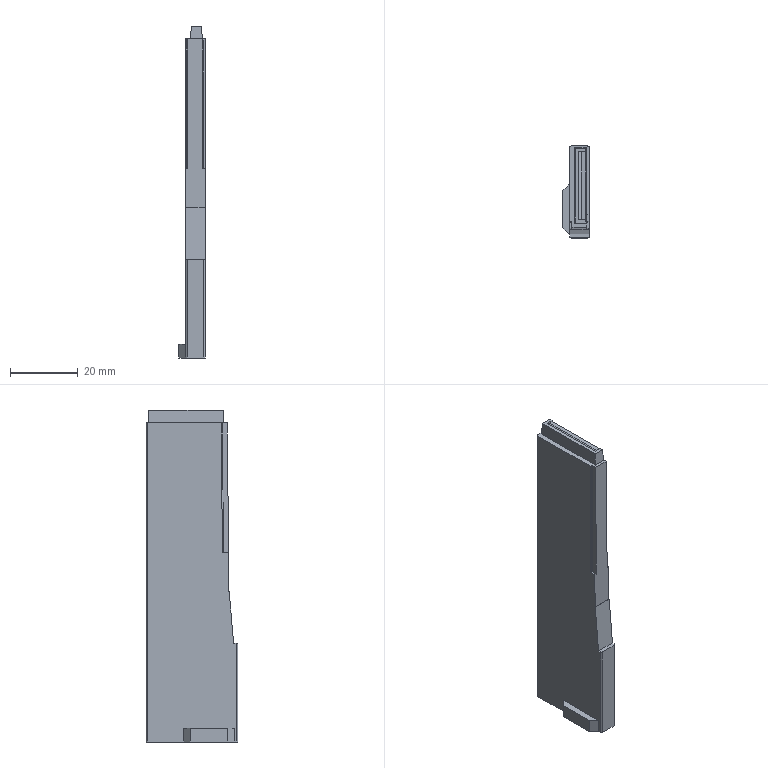Part | Creo | 1 solid | 40 faces | box 7.8 x 27 x 97.99 mm | volume 14019 mm3 | plane 33 | cylinder 7 | commonest cylinder face diameters 1 x4 0.603 x3
STEP:
#1=CARTESIAN_POINT('',(0.,0.,0.));
#2=DIRECTION('',(0.,0.,1.));
#3=DIRECTION('',(1.,0.,0.));
#4=AXIS2_PLACEMENT_3D('',#1,#2,#3);
#5=CARTESIAN_POINT('',(15.65,-83.325,43.9));
#6=VERTEX_POINT('',#5);
#7=CARTESIAN_POINT('',(15.65,-63.225,43.9));
#8=VERTEX_POINT('',#7);
#9=CARTESIAN_POINT('',(15.65,-83.325,43.9));
#10=DIRECTION('',(0.,1.,0.));
#11=VECTOR('',#10,20.1);
#12=LINE('',#9,#11);
#13=EDGE_CURVE('',#6,#8,#12,.T.);
#14=ORIENTED_EDGE('',*,*,#13,.T.);
#15=CARTESIAN_POINT('',(16.566,-63.256,43.548));
#16=VERTEX_POINT('',#15);
#17=CARTESIAN_POINT('',(15.65,-63.225,43.9));
#18=DIRECTION('',(0.9329,-0.03139,-0.3588));
#19=VECTOR('',#18,0.9817);
#20=LINE('',#17,#19);
#21=EDGE_CURVE('',#8,#16,#20,.T.);
#22=ORIENTED_EDGE('',*,*,#21,.T.);
#23=CARTESIAN_POINT('',(16.566,-83.294,43.548));
#24=VERTEX_POINT('',#23);
#25=CARTESIAN_POINT('',(16.566,-83.294,43.548));
#26=DIRECTION('',(0.,1.,0.));
#27=VECTOR('',#26,20.038);
#28=LINE('',#25,#27);
#29=EDGE_CURVE('',#24,#16,#28,.T.);
#30=ORIENTED_EDGE('',*,*,#29,.F.);
#31=CARTESIAN_POINT('',(15.65,-83.325,43.9));
#32=DIRECTION('',(0.9329,0.03139,-0.3588));
#33=VECTOR('',#32,0.9817);
#34=LINE('',#31,#33);
#35=EDGE_CURVE('',#6,#24,#34,.T.);
#36=ORIENTED_EDGE('',*,*,#35,.F.);
#37=EDGE_LOOP('',(#14,#22,#30,#36));
#38=FACE_OUTER_BOUND('',#37,.F.);
#39=CARTESIAN_POINT('',(15.65,-83.325,43.9));
#40=DIRECTION('',(-0.359,0.,-0.9333));
#41=DIRECTION('',(-0.9333,0.,0.359));
#42=AXIS2_PLACEMENT_3D('',#39,#40,#41);
#43=PLANE('',#42);
#44=ADVANCED_FACE('',(#38),#43,.F.);
#45=CARTESIAN_POINT('',(17.723,-62.246,43.9));
#46=VERTEX_POINT('',#45);
#47=CARTESIAN_POINT('',(14.671,-62.246,43.9));
#48=VERTEX_POINT('',#47);
#49=CARTESIAN_POINT('',(17.723,-62.246,43.9));
#50=DIRECTION('',(-1.,0.,0.));
#51=VECTOR('',#50,3.052);
#52=LINE('',#49,#51);
#53=EDGE_CURVE('',#46,#48,#52,.T.);
#54=ORIENTED_EDGE('',*,*,#53,.F.);
#55=CARTESIAN_POINT('',(17.723,-63.225,43.9));
#56=VERTEX_POINT('',#55);
#57=CARTESIAN_POINT('',(17.723,-63.225,43.9));
#58=DIRECTION('',(0.,1.,0.));
#59=VECTOR('',#58,0.9787);
#60=LINE('',#57,#59);
#61=EDGE_CURVE('',#56,#46,#60,.T.);
#62=ORIENTED_EDGE('',*,*,#61,.F.);
#63=CARTESIAN_POINT('',(15.65,-63.225,43.9));
#64=DIRECTION('',(1.,0.,0.));
#65=VECTOR('',#64,2.073);
#66=LINE('',#63,#65);
#67=EDGE_CURVE('',#8,#56,#66,.T.);
#68=ORIENTED_EDGE('',*,*,#67,.F.);
#69=ORIENTED_EDGE('',*,*,#13,.F.);
#70=CARTESIAN_POINT('',(17.723,-83.325,43.9));
#71=VERTEX_POINT('',#70);
#72=CARTESIAN_POINT('',(15.65,-83.325,43.9));
#73=DIRECTION('',(1.,0.,0.));
#74=VECTOR('',#73,2.073);
#75=LINE('',#72,#74);
#76=EDGE_CURVE('',#6,#71,#75,.T.);
#77=ORIENTED_EDGE('',*,*,#76,.T.);
#78=CARTESIAN_POINT('',(17.723,-84.304,43.9));
#79=VERTEX_POINT('',#78);
#80=CARTESIAN_POINT('',(17.723,-84.304,43.9));
#81=DIRECTION('',(0.,1.,0.));
#82=VECTOR('',#81,0.9787);
#83=LINE('',#80,#82);
#84=EDGE_CURVE('',#79,#71,#83,.T.);
#85=ORIENTED_EDGE('',*,*,#84,.F.);
#86=CARTESIAN_POINT('',(14.671,-84.304,43.9));
#87=VERTEX_POINT('',#86);
#88=CARTESIAN_POINT('',(14.671,-84.304,43.9));
#89=DIRECTION('',(1.,0.,0.));
#90=VECTOR('',#89,3.052);
#91=LINE('',#88,#90);
#92=EDGE_CURVE('',#87,#79,#91,.T.);
#93=ORIENTED_EDGE('',*,*,#92,.F.);
#94=CARTESIAN_POINT('',(14.671,-62.246,43.9));
#95=DIRECTION('',(0.,-1.,0.));
#96=VECTOR('',#95,22.057);
#97=LINE('',#94,#96);
#98=EDGE_CURVE('',#48,#87,#97,.T.);
#99=ORIENTED_EDGE('',*,*,#98,.F.);
#100=EDGE_LOOP('',(#54,#62,#68,#69,#77,#85,#93,#99));
#101=FACE_OUTER_BOUND('',#100,.F.);
#102=CARTESIAN_POINT('',(-46.35,-83.325,43.9));
#103=DIRECTION('',(0.,0.,-1.));
#104=DIRECTION('',(0.,-1.,0.));
#105=AXIS2_PLACEMENT_3D('',#102,#103,#104);
#106=PLANE('',#105);
#107=ADVANCED_FACE('',(#101),#106,.F.);
#108=CARTESIAN_POINT('',(17.722,-62.245,43.876));
#109=VERTEX_POINT('',#108);
#110=CARTESIAN_POINT('',(17.722,-62.245,43.876));
#111=DIRECTION('',(0.03485,-0.0523,0.998));
#112=VECTOR('',#111,0.02412);
#113=LINE('',#110,#112);
#114=EDGE_CURVE('',#109,#46,#113,.T.);
#115=ORIENTED_EDGE('',*,*,#114,.T.);
#116=ORIENTED_EDGE('',*,*,#53,.T.);
#117=CARTESIAN_POINT('',(14.471,-62.046,40.081));
#118=VERTEX_POINT('',#117);
#119=CARTESIAN_POINT('',(14.671,-62.246,43.9));
#120=DIRECTION('',(-0.05226,0.05226,-0.9973));
#121=VECTOR('',#120,3.829);
#122=LINE('',#119,#121);
#123=EDGE_CURVE('',#48,#118,#122,.T.);
#124=ORIENTED_EDGE('',*,*,#123,.T.);
#125=CARTESIAN_POINT('',(17.921,-62.046,40.081));
#126=VERTEX_POINT('',#125);
#127=CARTESIAN_POINT('',(14.471,-62.046,40.081));
#128=DIRECTION('',(1.,0.,0.));
#129=VECTOR('',#128,3.45);
#130=LINE('',#127,#129);
#131=EDGE_CURVE('',#118,#126,#130,.T.);
#132=ORIENTED_EDGE('',*,*,#131,.T.);
#133=CARTESIAN_POINT('',(17.921,-62.046,40.081));
#134=DIRECTION('',(-0.05226,-0.05226,0.9973));
#135=VECTOR('',#134,3.805);
#136=LINE('',#133,#135);
#137=EDGE_CURVE('',#126,#109,#136,.T.);
#138=ORIENTED_EDGE('',*,*,#137,.T.);
#139=EDGE_LOOP('',(#115,#116,#124,#132,#138));
#140=FACE_OUTER_BOUND('',#139,.F.);
#141=CARTESIAN_POINT('',(21.275,-62.22,43.398));
#142=DIRECTION('',(0.,0.9986,0.05234));
#143=DIRECTION('',(-1.,0.,0.));
#144=AXIS2_PLACEMENT_3D('',#141,#142,#143);
#145=PLANE('',#144);
#146=ADVANCED_FACE('',(#140),#145,.T.);
#147=ORIENTED_EDGE('',*,*,#61,.T.);
#148=ORIENTED_EDGE('',*,*,#114,.F.);
#149=CARTESIAN_POINT('',(17.722,-63.227,43.876));
#150=VERTEX_POINT('',#149);
#151=CARTESIAN_POINT('',(17.722,-63.227,43.876));
#152=DIRECTION('',(0.,1.,0.));
#153=VECTOR('',#152,0.982);
#154=LINE('',#151,#153);
#155=EDGE_CURVE('',#150,#109,#154,.T.);
#156=ORIENTED_EDGE('',*,*,#155,.F.);
#157=CARTESIAN_POINT('',(17.723,-63.225,43.9));
#158=DIRECTION('',(-0.03477,-0.0871,-0.9956));
#159=VECTOR('',#158,0.02417);
#160=LINE('',#157,#159);
#161=EDGE_CURVE('',#56,#150,#160,.T.);
#162=ORIENTED_EDGE('',*,*,#161,.F.);
#163=EDGE_LOOP('',(#147,#148,#156,#162));
#164=FACE_OUTER_BOUND('',#163,.F.);
#165=CARTESIAN_POINT('',(17.66,-62.152,42.091));
#166=DIRECTION('',(-0.9994,0.,0.0349));
#167=DIRECTION('',(0.0349,0.,0.9994));
#168=AXIS2_PLACEMENT_3D('',#165,#166,#167);
#169=PLANE('',#168);
#170=ADVANCED_FACE('',(#164),#169,.F.);
#171=CARTESIAN_POINT('',(17.74,-83.294,43.548));
#172=VERTEX_POINT('',#171);
#173=CARTESIAN_POINT('',(17.74,-63.256,43.548));
#174=VERTEX_POINT('',#173);
#175=CARTESIAN_POINT('',(17.74,-83.294,43.548));
#176=DIRECTION('',(0.,1.,0.));
#177=VECTOR('',#176,20.038);
#178=LINE('',#175,#177);
#179=EDGE_CURVE('',#172,#174,#178,.T.);
#180=ORIENTED_EDGE('',*,*,#179,.T.);
#181=CARTESIAN_POINT('',(17.722,-63.227,43.876));
#182=DIRECTION('',(0.05214,-0.08704,-0.9948));
#183=VECTOR('',#182,0.3299);
#184=LINE('',#181,#183);
#185=EDGE_CURVE('',#150,#174,#184,.T.);
#186=ORIENTED_EDGE('',*,*,#185,.F.);
#187=ORIENTED_EDGE('',*,*,#155,.T.);
#188=ORIENTED_EDGE('',*,*,#137,.F.);
#189=CARTESIAN_POINT('',(17.921,-84.504,40.081));
#190=VERTEX_POINT('',#189);
#191=CARTESIAN_POINT('',(17.921,-84.504,40.081));
#192=DIRECTION('',(0.,1.,0.));
#193=VECTOR('',#192,22.458);
#194=LINE('',#191,#193);
#195=EDGE_CURVE('',#190,#126,#194,.T.);
#196=ORIENTED_EDGE('',*,*,#195,.F.);
#197=CARTESIAN_POINT('',(17.722,-84.305,43.876));
#198=VERTEX_POINT('',#197);
#199=CARTESIAN_POINT('',(17.722,-84.305,43.876));
#200=DIRECTION('',(0.05226,-0.05226,-0.9973));
#201=VECTOR('',#200,3.805);
#202=LINE('',#199,#201);
#203=EDGE_CURVE('',#198,#190,#202,.T.);
#204=ORIENTED_EDGE('',*,*,#203,.F.);
#205=CARTESIAN_POINT('',(17.722,-83.323,43.876));
#206=VERTEX_POINT('',#205);
#207=CARTESIAN_POINT('',(17.722,-84.305,43.876));
#208=DIRECTION('',(0.,1.,0.));
#209=VECTOR('',#208,0.982);
#210=LINE('',#207,#209);
#211=EDGE_CURVE('',#198,#206,#210,.T.);
#212=ORIENTED_EDGE('',*,*,#211,.T.);
#213=CARTESIAN_POINT('',(17.74,-83.294,43.548));
#214=DIRECTION('',(-0.05214,-0.08704,0.9948));
#215=VECTOR('',#214,0.3299);
#216=LINE('',#213,#215);
#217=EDGE_CURVE('',#172,#206,#216,.T.);
#218=ORIENTED_EDGE('',*,*,#217,.F.);
#219=EDGE_LOOP('',(#180,#186,#187,#188,#196,#204,#212,#218));
#220=FACE_OUTER_BOUND('',#219,.F.);
#221=CARTESIAN_POINT('',(17.747,-90.96,43.402));
#222=DIRECTION('',(-0.9986,0.,-0.05234));
#223=DIRECTION('',(0.,-1.,0.));
#224=AXIS2_PLACEMENT_3D('',#221,#222,#223);
#225=PLANE('',#224);
#226=ADVANCED_FACE('',(#220),#225,.F.);
#227=ORIENTED_EDGE('',*,*,#29,.T.);
#228=CARTESIAN_POINT('',(16.566,-63.256,43.548));
#229=DIRECTION('',(1.,0.,0.));
#230=VECTOR('',#229,1.174);
#231=LINE('',#228,#230);
#232=EDGE_CURVE('',#16,#174,#231,.T.);
#233=ORIENTED_EDGE('',*,*,#232,.T.);
#234=ORIENTED_EDGE('',*,*,#179,.F.);
#235=CARTESIAN_POINT('',(16.566,-83.294,43.548));
#236=DIRECTION('',(1.,0.,0.));
#237=VECTOR('',#236,1.174);
#238=LINE('',#235,#237);
#239=EDGE_CURVE('',#24,#172,#238,.T.);
#240=ORIENTED_EDGE('',*,*,#239,.F.);
#241=EDGE_LOOP('',(#227,#233,#234,#240));
#242=FACE_OUTER_BOUND('',#241,.F.);
#243=CARTESIAN_POINT('',(16.956,-83.325,43.548));
#244=DIRECTION('',(0.,0.,-1.));
#245=DIRECTION('',(-1.,0.,0.));
#246=AXIS2_PLACEMENT_3D('',#243,#244,#245);
#247=PLANE('',#246);
#248=ADVANCED_FACE('',(#242),#247,.F.);
#249=ORIENTED_EDGE('',*,*,#67,.T.);
#250=ORIENTED_EDGE('',*,*,#161,.T.);
#251=ORIENTED_EDGE('',*,*,#185,.T.);
#252=ORIENTED_EDGE('',*,*,#232,.F.);
#253=ORIENTED_EDGE('',*,*,#21,.F.);
#254=EDGE_LOOP('',(#249,#250,#251,#252,#253));
#255=FACE_OUTER_BOUND('',#254,.F.);
#256=CARTESIAN_POINT('',(-0.07825,-63.225,43.9));
#257=DIRECTION('',(0.,0.9962,-0.08716));
#258=DIRECTION('',(0.,-0.08716,-0.9962));
#259=AXIS2_PLACEMENT_3D('',#256,#257,#258);
#260=PLANE('',#259);
#261=ADVANCED_FACE('',(#255),#260,.F.);
#262=CARTESIAN_POINT('',(17.723,-83.325,43.9));
#263=DIRECTION('',(-0.03477,0.0871,-0.9956));
#264=VECTOR('',#263,0.02417);
#265=LINE('',#262,#264);
#266=EDGE_CURVE('',#71,#206,#265,.T.);
#267=ORIENTED_EDGE('',*,*,#266,.F.);
#268=ORIENTED_EDGE('',*,*,#76,.F.);
#269=ORIENTED_EDGE('',*,*,#35,.T.);
#270=ORIENTED_EDGE('',*,*,#239,.T.);
#271=ORIENTED_EDGE('',*,*,#217,.T.);
#272=EDGE_LOOP('',(#267,#268,#269,#270,#271));
#273=FACE_OUTER_BOUND('',#272,.F.);
#274=CARTESIAN_POINT('',(-0.07825,-83.325,43.9));
#275=DIRECTION('',(0.,-0.9962,-0.08716));
#276=DIRECTION('',(0.,-0.08716,0.9962));
#277=AXIS2_PLACEMENT_3D('',#274,#275,#276);
#278=PLANE('',#277);
#279=ADVANCED_FACE('',(#273),#278,.F.);
#280=ORIENTED_EDGE('',*,*,#84,.T.);
#281=ORIENTED_EDGE('',*,*,#266,.T.);
#282=ORIENTED_EDGE('',*,*,#211,.F.);
#283=CARTESIAN_POINT('',(17.722,-84.305,43.876));
#284=DIRECTION('',(0.03485,0.0523,0.998));
#285=VECTOR('',#284,0.02412);
#286=LINE('',#283,#285);
#287=EDGE_CURVE('',#198,#79,#286,.T.);
#288=ORIENTED_EDGE('',*,*,#287,.T.);
#289=EDGE_LOOP('',(#280,#281,#282,#288));
#290=FACE_OUTER_BOUND('',#289,.F.);
#291=CARTESIAN_POINT('',(17.66,-88.149,42.091));
#292=DIRECTION('',(-0.9994,0.,0.0349));
#293=DIRECTION('',(0.0349,0.,0.9994));
#294=AXIS2_PLACEMENT_3D('',#291,#292,#293);
#295=PLANE('',#294);
#296=ADVANCED_FACE('',(#290),#295,.F.);
#297=ORIENTED_EDGE('',*,*,#203,.T.);
#298=CARTESIAN_POINT('',(14.471,-84.504,40.081));
#299=VERTEX_POINT('',#298);
#300=CARTESIAN_POINT('',(17.921,-84.504,40.081));
#301=DIRECTION('',(-1.,0.,0.));
#302=VECTOR('',#301,3.45);
#303=LINE('',#300,#302);
#304=EDGE_CURVE('',#190,#299,#303,.T.);
#305=ORIENTED_EDGE('',*,*,#304,.T.);
#306=CARTESIAN_POINT('',(14.671,-84.304,43.9));
#307=DIRECTION('',(-0.05226,-0.05226,-0.9973));
#308=VECTOR('',#307,3.829);
#309=LINE('',#306,#308);
#310=EDGE_CURVE('',#87,#299,#309,.T.);
#311=ORIENTED_EDGE('',*,*,#310,.F.);
#312=ORIENTED_EDGE('',*,*,#92,.T.);
#313=ORIENTED_EDGE('',*,*,#287,.F.);
#314=EDGE_LOOP('',(#297,#305,#311,#312,#313));
#315=FACE_OUTER_BOUND('',#314,.F.);
#316=CARTESIAN_POINT('',(11.03,-84.33,43.398));
#317=DIRECTION('',(0.,-0.9986,0.05234));
#318=DIRECTION('',(1.,0.,0.));
#319=AXIS2_PLACEMENT_3D('',#316,#317,#318);
#320=PLANE('',#319);
#321=ADVANCED_FACE('',(#315),#320,.T.);
#322=CARTESIAN_POINT('',(18.797,-81.805,40.081));
#323=VERTEX_POINT('',#322);
#324=CARTESIAN_POINT('',(18.797,-62.049,40.081));
#325=VERTEX_POINT('',#324);
#326=CARTESIAN_POINT('',(18.797,-81.805,40.081));
#327=DIRECTION('',(0.,1.,0.));
#328=VECTOR('',#327,19.756);
#329=LINE('',#326,#328);
#330=EDGE_CURVE('',#323,#325,#329,.T.);
#331=ORIENTED_EDGE('',*,*,#330,.F.);
#332=CARTESIAN_POINT('',(18.301,-81.805,40.081));
#333=VERTEX_POINT('',#332);
#334=CARTESIAN_POINT('',(18.797,-81.805,40.081));
#335=DIRECTION('',(-1.,0.,0.));
#336=VECTOR('',#335,0.4964);
#337=LINE('',#334,#336);
#338=EDGE_CURVE('',#323,#333,#337,.T.);
#339=ORIENTED_EDGE('',*,*,#338,.T.);
#340=CARTESIAN_POINT('',(17.999,-82.107,40.081));
#341=VERTEX_POINT('',#340);
#342=CARTESIAN_POINT('',(18.2,-81.805,40.081));
#343=CARTESIAN_POINT('',(18.076,-81.881,40.081));
#344=CARTESIAN_POINT('',(17.999,-82.006,40.081));
#345=B_SPLINE_CURVE_WITH_KNOTS('',3,(#332,#342,#343,#344,#340),.UNSPECIFIED.,.F.,.F.,(4,1,4),(0.,0.5,1.),.UNSPECIFIED.);
#346=EDGE_CURVE('',#333,#341,#345,.T.);
#347=ORIENTED_EDGE('',*,*,#346,.T.);
#348=CARTESIAN_POINT('',(17.999,-85.486,40.081));
#349=VERTEX_POINT('',#348);
#350=CARTESIAN_POINT('',(17.999,-82.107,40.081));
#351=DIRECTION('',(0.,-1.,0.));
#352=VECTOR('',#351,3.379);
#353=LINE('',#350,#352);
#354=EDGE_CURVE('',#341,#349,#353,.T.);
#355=ORIENTED_EDGE('',*,*,#354,.T.);
#356=CARTESIAN_POINT('',(13.703,-85.486,40.081));
#357=VERTEX_POINT('',#356);
#358=CARTESIAN_POINT('',(13.703,-85.486,40.081));
#359=DIRECTION('',(1.,0.,0.));
#360=VECTOR('',#359,4.297);
#361=LINE('',#358,#360);
#362=EDGE_CURVE('',#357,#349,#361,.T.);
#363=ORIENTED_EDGE('',*,*,#362,.F.);
#364=CARTESIAN_POINT('',(13.703,-84.117,40.081));
#365=VERTEX_POINT('',#364);
#366=CARTESIAN_POINT('',(13.703,-85.486,40.081));
#367=DIRECTION('',(0.,1.,0.));
#368=VECTOR('',#367,1.369);
#369=LINE('',#366,#368);
#370=EDGE_CURVE('',#357,#365,#369,.T.);
#371=ORIENTED_EDGE('',*,*,#370,.T.);
#372=CARTESIAN_POINT('',(13.401,-83.815,40.081));
#373=VERTEX_POINT('',#372);
#374=CARTESIAN_POINT('',(13.703,-84.117,40.081));
#375=CARTESIAN_POINT('',(13.703,-84.016,40.081));
#376=CARTESIAN_POINT('',(13.626,-83.891,40.081));
#377=CARTESIAN_POINT('',(13.502,-83.815,40.081));
#378=B_SPLINE_CURVE_WITH_KNOTS('',3,(#374,#375,#376,#377,#372),.UNSPECIFIED.,.F.,.F.,(4,1,4),(0.,0.5,1.),.UNSPECIFIED.);
#379=EDGE_CURVE('',#365,#373,#378,.T.);
#380=ORIENTED_EDGE('',*,*,#379,.T.);
#381=CARTESIAN_POINT('',(12.997,-83.815,40.081));
#382=VERTEX_POINT('',#381);
#383=CARTESIAN_POINT('',(12.997,-83.815,40.081));
#384=DIRECTION('',(1.,0.,0.));
#385=VECTOR('',#384,0.4037);
#386=LINE('',#383,#385);
#387=EDGE_CURVE('',#382,#373,#386,.T.);
#388=ORIENTED_EDGE('',*,*,#387,.F.);
#389=CARTESIAN_POINT('',(12.997,-62.049,40.081));
#390=VERTEX_POINT('',#389);
#391=CARTESIAN_POINT('',(12.997,-62.049,40.081));
#392=DIRECTION('',(0.,-1.,0.));
#393=VECTOR('',#392,21.766);
#394=LINE('',#391,#393);
#395=EDGE_CURVE('',#390,#382,#394,.T.);
#396=ORIENTED_EDGE('',*,*,#395,.F.);
#397=CARTESIAN_POINT('',(13.497,-61.549,40.081));
#398=VERTEX_POINT('',#397);
#399=CARTESIAN_POINT('',(13.497,-62.049,40.081));
#400=DIRECTION('',(0.,0.,1.));
#401=DIRECTION('',(0.,1.,0.));
#402=AXIS2_PLACEMENT_3D('',#399,#400,#401);
#403=CIRCLE('',#402,0.5);
#404=EDGE_CURVE('',#398,#390,#403,.T.);
#405=ORIENTED_EDGE('',*,*,#404,.F.);
#406=CARTESIAN_POINT('',(18.297,-61.549,40.081));
#407=VERTEX_POINT('',#406);
#408=CARTESIAN_POINT('',(18.297,-61.549,40.081));
#409=DIRECTION('',(-1.,0.,0.));
#410=VECTOR('',#409,4.8);
#411=LINE('',#408,#410);
#412=EDGE_CURVE('',#407,#398,#411,.T.);
#413=ORIENTED_EDGE('',*,*,#412,.F.);
#414=CARTESIAN_POINT('',(18.297,-62.049,40.081));
#415=DIRECTION('',(0.,0.,1.));
#416=DIRECTION('',(1.,0.,0.));
#417=AXIS2_PLACEMENT_3D('',#414,#415,#416);
#418=CIRCLE('',#417,0.5);
#419=EDGE_CURVE('',#325,#407,#418,.T.);
#420=ORIENTED_EDGE('',*,*,#419,.F.);
#421=EDGE_LOOP('',(#331,#339,#347,#355,#363,#371,#380,#388,#396,#405,#413,#420));
#422=FACE_OUTER_BOUND('',#421,.F.);
#423=ORIENTED_EDGE('',*,*,#195,.T.);
#424=ORIENTED_EDGE('',*,*,#131,.F.);
#425=CARTESIAN_POINT('',(14.471,-84.504,40.081));
#426=DIRECTION('',(0.,1.,0.));
#427=VECTOR('',#426,22.458);
#428=LINE('',#425,#427);
#429=EDGE_CURVE('',#299,#118,#428,.T.);
#430=ORIENTED_EDGE('',*,*,#429,.F.);
#431=ORIENTED_EDGE('',*,*,#304,.F.);
#432=EDGE_LOOP('',(#423,#424,#430,#431));
#433=FACE_BOUND('',#432,.F.);
#434=CARTESIAN_POINT('',(-17.817,-88.35,40.081));
#435=DIRECTION('',(0.,0.,1.));
#436=DIRECTION('',(-1.,0.,0.));
#437=AXIS2_PLACEMENT_3D('',#434,#435,#436);
#438=PLANE('',#437);
#439=ADVANCED_FACE('',(#422,#433),#438,.T.);
#440=ORIENTED_EDGE('',*,*,#429,.T.);
#441=ORIENTED_EDGE('',*,*,#123,.F.);
#442=ORIENTED_EDGE('',*,*,#98,.T.);
#443=ORIENTED_EDGE('',*,*,#310,.T.);
#444=EDGE_LOOP('',(#440,#441,#442,#443));
#445=FACE_OUTER_BOUND('',#444,.F.);
#446=CARTESIAN_POINT('',(14.645,-58.605,43.398));
#447=DIRECTION('',(-0.9986,0.,0.05234));
#448=DIRECTION('',(0.,-1.,0.));
#449=AXIS2_PLACEMENT_3D('',#446,#447,#448);
#450=PLANE('',#449);
#451=ADVANCED_FACE('',(#445),#450,.T.);
#452=CARTESIAN_POINT('',(18.797,-87.347,-24.967));
#453=VERTEX_POINT('',#452);
#454=CARTESIAN_POINT('',(18.797,-88.049,-24.967));
#455=VERTEX_POINT('',#454);
#456=CARTESIAN_POINT('',(18.797,-87.347,-24.967));
#457=DIRECTION('',(0.,-1.,0.));
#458=VECTOR('',#457,0.7016);
#459=LINE('',#456,#458);
#460=EDGE_CURVE('',#453,#455,#459,.T.);
#461=ORIENTED_EDGE('',*,*,#460,.F.);
#462=CARTESIAN_POINT('',(18.797,-86.017,-9.767));
#463=VERTEX_POINT('',#462);
#464=CARTESIAN_POINT('',(18.797,-86.017,-9.767));
#465=DIRECTION('',(0.,-0.08716,-0.9962));
#466=VECTOR('',#465,15.258);
#467=LINE('',#464,#466);
#468=EDGE_CURVE('',#463,#453,#467,.T.);
#469=ORIENTED_EDGE('',*,*,#468,.F.);
#470=CARTESIAN_POINT('',(18.797,-85.921,-9.767));
#471=VERTEX_POINT('',#470);
#472=CARTESIAN_POINT('',(18.797,-85.921,-9.767));
#473=DIRECTION('',(0.,-1.,0.));
#474=VECTOR('',#473,0.09668);
#475=LINE('',#472,#474);
#476=EDGE_CURVE('',#471,#463,#475,.T.);
#477=ORIENTED_EDGE('',*,*,#476,.F.);
#478=CARTESIAN_POINT('',(18.797,-85.82,1.79));
#479=VERTEX_POINT('',#478);
#480=CARTESIAN_POINT('',(18.797,-85.82,1.79));
#481=DIRECTION('',(0.,-0.008727,-1.));
#482=VECTOR('',#481,11.558);
#483=LINE('',#480,#482);
#484=EDGE_CURVE('',#479,#471,#483,.T.);
#485=ORIENTED_EDGE('',*,*,#484,.F.);
#486=CARTESIAN_POINT('',(18.797,-83.949,1.79));
#487=VERTEX_POINT('',#486);
#488=CARTESIAN_POINT('',(18.797,-83.949,1.79));
#489=DIRECTION('',(0.,-1.,0.));
#490=VECTOR('',#489,1.871);
#491=LINE('',#488,#490);
#492=EDGE_CURVE('',#487,#479,#491,.T.);
#493=ORIENTED_EDGE('',*,*,#492,.F.);
#494=CARTESIAN_POINT('',(18.797,-83.828,36.563));
#495=VERTEX_POINT('',#494);
#496=CARTESIAN_POINT('',(18.797,-83.828,36.563));
#497=DIRECTION('',(0.,-0.003491,-1.));
#498=VECTOR('',#497,34.773);
#499=LINE('',#496,#498);
#500=EDGE_CURVE('',#495,#487,#499,.T.);
#501=ORIENTED_EDGE('',*,*,#500,.F.);
#502=CARTESIAN_POINT('',(18.797,-81.817,36.563));
#503=VERTEX_POINT('',#502);
#504=CARTESIAN_POINT('',(18.797,-83.828,36.563));
#505=DIRECTION('',(0.,1.,0.));
#506=VECTOR('',#505,2.01);
#507=LINE('',#504,#506);
#508=EDGE_CURVE('',#495,#503,#507,.T.);
#509=ORIENTED_EDGE('',*,*,#508,.T.);
#510=CARTESIAN_POINT('',(18.797,-81.805,40.081));
#511=DIRECTION('',(0.,-0.003491,-1.));
#512=VECTOR('',#511,3.518);
#513=LINE('',#510,#512);
#514=EDGE_CURVE('',#323,#503,#513,.T.);
#515=ORIENTED_EDGE('',*,*,#514,.F.);
#516=ORIENTED_EDGE('',*,*,#330,.T.);
#517=CARTESIAN_POINT('',(18.797,-62.049,-54.09));
#518=VERTEX_POINT('',#517);
#519=CARTESIAN_POINT('',(18.797,-62.049,40.081));
#520=DIRECTION('',(0.,0.,-1.));
#521=VECTOR('',#520,94.171);
#522=LINE('',#519,#521);
#523=EDGE_CURVE('',#325,#518,#522,.T.);
#524=ORIENTED_EDGE('',*,*,#523,.T.);
#525=CARTESIAN_POINT('',(18.797,-88.049,-54.09));
#526=VERTEX_POINT('',#525);
#527=CARTESIAN_POINT('',(18.797,-62.049,-54.09));
#528=DIRECTION('',(0.,-1.,0.));
#529=VECTOR('',#528,26.);
#530=LINE('',#527,#529);
#531=EDGE_CURVE('',#518,#526,#530,.T.);
#532=ORIENTED_EDGE('',*,*,#531,.T.);
#533=CARTESIAN_POINT('',(18.797,-88.049,-54.09));
#534=DIRECTION('',(0.,0.,1.));
#535=VECTOR('',#534,29.123);
#536=LINE('',#533,#535);
#537=EDGE_CURVE('',#526,#455,#536,.T.);
#538=ORIENTED_EDGE('',*,*,#537,.T.);
#539=EDGE_LOOP('',(#461,#469,#477,#485,#493,#501,#509,#515,#516,#524,#532,#538));
#540=FACE_OUTER_BOUND('',#539,.F.);
#541=CARTESIAN_POINT('',(18.797,-88.549,68.91));
#542=DIRECTION('',(-1.,0.,0.));
#543=DIRECTION('',(0.,0.,1.));
#544=AXIS2_PLACEMENT_3D('',#541,#542,#543);
#545=PLANE('',#544);
#546=ADVANCED_FACE('',(#540),#545,.F.);
#547=CARTESIAN_POINT('',(18.297,-88.549,-24.967));
#548=VERTEX_POINT('',#547);
#549=CARTESIAN_POINT('',(13.497,-88.549,-24.967));
#550=VERTEX_POINT('',#549);
#551=CARTESIAN_POINT('',(18.297,-88.549,-24.967));
#552=DIRECTION('',(-1.,0.,0.));
#553=VECTOR('',#552,4.8);
#554=LINE('',#551,#553);
#555=EDGE_CURVE('',#548,#550,#554,.T.);
#556=ORIENTED_EDGE('',*,*,#555,.T.);
#557=CARTESIAN_POINT('',(12.997,-88.049,-24.967));
#558=VERTEX_POINT('',#557);
#559=CARTESIAN_POINT('',(13.497,-88.049,-24.967));
#560=DIRECTION('',(0.,0.,1.));
#561=DIRECTION('',(-1.,0.,0.));
#562=AXIS2_PLACEMENT_3D('',#559,#560,#561);
#563=CIRCLE('',#562,0.5);
#564=EDGE_CURVE('',#558,#550,#563,.T.);
#565=ORIENTED_EDGE('',*,*,#564,.F.);
#566=CARTESIAN_POINT('',(12.997,-87.347,-24.967));
#567=VERTEX_POINT('',#566);
#568=CARTESIAN_POINT('',(12.997,-88.049,-24.967));
#569=DIRECTION('',(0.,1.,0.));
#570=VECTOR('',#569,0.7016);
#571=LINE('',#568,#570);
#572=EDGE_CURVE('',#558,#567,#571,.T.);
#573=ORIENTED_EDGE('',*,*,#572,.T.);
#574=CARTESIAN_POINT('',(12.997,-87.347,-24.967));
#575=DIRECTION('',(1.,0.,0.));
#576=VECTOR('',#575,5.8);
#577=LINE('',#574,#576);
#578=EDGE_CURVE('',#567,#453,#577,.T.);
#579=ORIENTED_EDGE('',*,*,#578,.T.);
#580=ORIENTED_EDGE('',*,*,#460,.T.);
#581=CARTESIAN_POINT('',(18.297,-88.049,-24.967));
#582=DIRECTION('',(0.,0.,1.));
#583=DIRECTION('',(0.,-1.,0.));
#584=AXIS2_PLACEMENT_3D('',#581,#582,#583);
#585=CIRCLE('',#584,0.5);
#586=EDGE_CURVE('',#548,#455,#585,.T.);
#587=ORIENTED_EDGE('',*,*,#586,.F.);
#588=EDGE_LOOP('',(#556,#565,#573,#579,#580,#587));
#589=FACE_OUTER_BOUND('',#588,.F.);
#590=CARTESIAN_POINT('',(-0.07825,-93.918,-24.967));
#591=DIRECTION('',(0.,0.,-1.));
#592=DIRECTION('',(0.,1.,0.));
#593=AXIS2_PLACEMENT_3D('',#590,#591,#592);
#594=PLANE('',#593);
#595=ADVANCED_FACE('',(#589),#594,.F.);
#596=CARTESIAN_POINT('',(18.297,-88.549,-54.09));
#597=VERTEX_POINT('',#596);
#598=CARTESIAN_POINT('',(13.497,-88.549,-54.09));
#599=VERTEX_POINT('',#598);
#600=CARTESIAN_POINT('',(18.297,-88.549,-54.09));
#601=DIRECTION('',(-1.,0.,0.));
#602=VECTOR('',#601,4.8);
#603=LINE('',#600,#602);
#604=EDGE_CURVE('',#597,#599,#603,.T.);
#605=ORIENTED_EDGE('',*,*,#604,.T.);
#606=CARTESIAN_POINT('',(13.497,-88.549,-54.09));
#607=DIRECTION('',(0.,0.,1.));
#608=VECTOR('',#607,29.123);
#609=LINE('',#606,#608);
#610=EDGE_CURVE('',#599,#550,#609,.T.);
#611=ORIENTED_EDGE('',*,*,#610,.T.);
#612=ORIENTED_EDGE('',*,*,#555,.F.);
#613=CARTESIAN_POINT('',(18.297,-88.549,-24.967));
#614=DIRECTION('',(0.,0.,-1.));
#615=VECTOR('',#614,29.123);
#616=LINE('',#613,#615);
#617=EDGE_CURVE('',#548,#597,#616,.T.);
#618=ORIENTED_EDGE('',*,*,#617,.T.);
#619=EDGE_LOOP('',(#605,#611,#612,#618));
#620=FACE_OUTER_BOUND('',#619,.F.);
#621=CARTESIAN_POINT('',(12.997,-88.549,68.91));
#622=DIRECTION('',(0.,1.,0.));
#623=DIRECTION('',(0.,0.,1.));
#624=AXIS2_PLACEMENT_3D('',#621,#622,#623);
#625=PLANE('',#624);
#626=ADVANCED_FACE('',(#620),#625,.F.);
#627=CARTESIAN_POINT('',(12.997,-88.049,-54.09));
#628=VERTEX_POINT('',#627);
#629=CARTESIAN_POINT('',(12.997,-87.549,-54.09));
#630=VERTEX_POINT('',#629);
#631=CARTESIAN_POINT('',(12.997,-88.049,-54.09));
#632=DIRECTION('',(0.,1.,0.));
#633=VECTOR('',#632,0.5);
#634=LINE('',#631,#633);
#635=EDGE_CURVE('',#628,#630,#634,.T.);
#636=ORIENTED_EDGE('',*,*,#635,.F.);
#637=CARTESIAN_POINT('',(13.497,-88.049,-54.09));
#638=DIRECTION('',(0.,0.,-1.));
#639=DIRECTION('',(0.,-1.,0.));
#640=AXIS2_PLACEMENT_3D('',#637,#638,#639);
#641=CIRCLE('',#640,0.5);
#642=EDGE_CURVE('',#599,#628,#641,.T.);
#643=ORIENTED_EDGE('',*,*,#642,.F.);
#644=ORIENTED_EDGE('',*,*,#604,.F.);
#645=CARTESIAN_POINT('',(18.297,-88.049,-54.09));
#646=DIRECTION('',(0.,0.,-1.));
#647=DIRECTION('',(1.,0.,0.));
#648=AXIS2_PLACEMENT_3D('',#645,#646,#647);
#649=CIRCLE('',#648,0.5);
#650=EDGE_CURVE('',#526,#597,#649,.T.);
#651=ORIENTED_EDGE('',*,*,#650,.F.);
#652=ORIENTED_EDGE('',*,*,#531,.F.);
#653=CARTESIAN_POINT('',(18.297,-61.549,-54.09));
#654=VERTEX_POINT('',#653);
#655=CARTESIAN_POINT('',(18.297,-62.049,-54.09));
#656=DIRECTION('',(0.,0.,-1.));
#657=DIRECTION('',(0.,1.,0.));
#658=AXIS2_PLACEMENT_3D('',#655,#656,#657);
#659=CIRCLE('',#658,0.5);
#660=EDGE_CURVE('',#654,#518,#659,.T.);
#661=ORIENTED_EDGE('',*,*,#660,.F.);
#662=CARTESIAN_POINT('',(13.497,-61.549,-54.09));
#663=VERTEX_POINT('',#662);
#664=CARTESIAN_POINT('',(13.497,-61.549,-54.09));
#665=DIRECTION('',(1.,0.,0.));
#666=VECTOR('',#665,4.8);
#667=LINE('',#664,#666);
#668=EDGE_CURVE('',#663,#654,#667,.T.);
#669=ORIENTED_EDGE('',*,*,#668,.F.);
#670=CARTESIAN_POINT('',(12.997,-62.049,-54.09));
#671=VERTEX_POINT('',#670);
#672=CARTESIAN_POINT('',(13.497,-62.049,-54.09));
#673=DIRECTION('',(0.,0.,-1.));
#674=DIRECTION('',(-1.,0.,0.));
#675=AXIS2_PLACEMENT_3D('',#672,#673,#674);
#676=CIRCLE('',#675,0.5);
#677=EDGE_CURVE('',#671,#663,#676,.T.);
#678=ORIENTED_EDGE('',*,*,#677,.F.);
#679=CARTESIAN_POINT('',(12.997,-72.549,-54.09));
#680=VERTEX_POINT('',#679);
#681=CARTESIAN_POINT('',(12.997,-72.549,-54.09));
#682=DIRECTION('',(0.,1.,0.));
#683=VECTOR('',#682,10.5);
#684=LINE('',#681,#683);
#685=EDGE_CURVE('',#680,#671,#684,.T.);
#686=ORIENTED_EDGE('',*,*,#685,.F.);
#687=CARTESIAN_POINT('',(10.997,-74.549,-54.09));
#688=VERTEX_POINT('',#687);
#689=CARTESIAN_POINT('',(10.997,-74.549,-54.09));
#690=DIRECTION('',(0.7071,0.7071,0.));
#691=VECTOR('',#690,2.828);
#692=LINE('',#689,#691);
#693=EDGE_CURVE('',#688,#680,#692,.T.);
#694=ORIENTED_EDGE('',*,*,#693,.F.);
#695=CARTESIAN_POINT('',(10.997,-85.549,-54.09));
#696=VERTEX_POINT('',#695);
#697=CARTESIAN_POINT('',(10.997,-85.549,-54.09));
#698=DIRECTION('',(0.,1.,0.));
#699=VECTOR('',#698,11.);
#700=LINE('',#697,#699);
#701=EDGE_CURVE('',#696,#688,#700,.T.);
#702=ORIENTED_EDGE('',*,*,#701,.F.);
#703=CARTESIAN_POINT('',(12.997,-87.549,-54.09));
#704=DIRECTION('',(-0.7071,0.7071,0.));
#705=VECTOR('',#704,2.828);
#706=LINE('',#703,#705);
#707=EDGE_CURVE('',#630,#696,#706,.T.);
#708=ORIENTED_EDGE('',*,*,#707,.F.);
#709=EDGE_LOOP('',(#636,#643,#644,#651,#652,#661,#669,#678,#686,#694,#702,#708));
#710=FACE_OUTER_BOUND('',#709,.F.);
#711=CARTESIAN_POINT('',(0.,0.,-54.09));
#712=DIRECTION('',(0.,0.,-1.));
#713=DIRECTION('',(-1.,0.,0.));
#714=AXIS2_PLACEMENT_3D('',#711,#712,#713);
#715=PLANE('',#714);
#716=ADVANCED_FACE('',(#710),#715,.T.);
#717=CARTESIAN_POINT('',(12.997,-87.549,-50.09));
#718=VERTEX_POINT('',#717);
#719=CARTESIAN_POINT('',(12.997,-72.549,-50.09));
#720=VERTEX_POINT('',#719);
#721=CARTESIAN_POINT('',(12.997,-87.549,-50.09));
#722=DIRECTION('',(0.,1.,0.));
#723=VECTOR('',#722,15.);
#724=LINE('',#721,#723);
#725=EDGE_CURVE('',#718,#720,#724,.T.);
#726=ORIENTED_EDGE('',*,*,#725,.T.);
#727=CARTESIAN_POINT('',(12.997,-72.549,-50.09));
#728=DIRECTION('',(0.,0.,-1.));
#729=VECTOR('',#728,4.);
#730=LINE('',#727,#729);
#731=EDGE_CURVE('',#720,#680,#730,.T.);
#732=ORIENTED_EDGE('',*,*,#731,.T.);
#733=ORIENTED_EDGE('',*,*,#685,.T.);
#734=CARTESIAN_POINT('',(12.997,-62.049,-54.09));
#735=DIRECTION('',(0.,0.,1.));
#736=VECTOR('',#735,94.171);
#737=LINE('',#734,#736);
#738=EDGE_CURVE('',#671,#390,#737,.T.);
#739=ORIENTED_EDGE('',*,*,#738,.T.);
#740=ORIENTED_EDGE('',*,*,#395,.T.);
#741=CARTESIAN_POINT('',(12.997,-83.949,1.79));
#742=VERTEX_POINT('',#741);
#743=CARTESIAN_POINT('',(12.997,-83.949,1.79));
#744=DIRECTION('',(0.,0.003491,1.));
#745=VECTOR('',#744,38.291);
#746=LINE('',#743,#745);
#747=EDGE_CURVE('',#742,#382,#746,.T.);
#748=ORIENTED_EDGE('',*,*,#747,.F.);
#749=CARTESIAN_POINT('',(12.997,-85.82,1.79));
#750=VERTEX_POINT('',#749);
#751=CARTESIAN_POINT('',(12.997,-85.82,1.79));
#752=DIRECTION('',(0.,1.,0.));
#753=VECTOR('',#752,1.871);
#754=LINE('',#751,#753);
#755=EDGE_CURVE('',#750,#742,#754,.T.);
#756=ORIENTED_EDGE('',*,*,#755,.F.);
#757=CARTESIAN_POINT('',(12.997,-85.921,-9.767));
#758=VERTEX_POINT('',#757);
#759=CARTESIAN_POINT('',(12.997,-85.921,-9.767));
#760=DIRECTION('',(0.,0.008727,1.));
#761=VECTOR('',#760,11.558);
#762=LINE('',#759,#761);
#763=EDGE_CURVE('',#758,#750,#762,.T.);
#764=ORIENTED_EDGE('',*,*,#763,.F.);
#765=CARTESIAN_POINT('',(12.997,-86.017,-9.767));
#766=VERTEX_POINT('',#765);
#767=CARTESIAN_POINT('',(12.997,-86.017,-9.767));
#768=DIRECTION('',(0.,1.,0.));
#769=VECTOR('',#768,0.09668);
#770=LINE('',#767,#769);
#771=EDGE_CURVE('',#766,#758,#770,.T.);
#772=ORIENTED_EDGE('',*,*,#771,.F.);
#773=CARTESIAN_POINT('',(12.997,-87.347,-24.967));
#774=DIRECTION('',(0.,0.08716,0.9962));
#775=VECTOR('',#774,15.258);
#776=LINE('',#773,#775);
#777=EDGE_CURVE('',#567,#766,#776,.T.);
#778=ORIENTED_EDGE('',*,*,#777,.F.);
#779=ORIENTED_EDGE('',*,*,#572,.F.);
#780=CARTESIAN_POINT('',(12.997,-88.049,-24.967));
#781=DIRECTION('',(0.,0.,-1.));
#782=VECTOR('',#781,29.123);
#783=LINE('',#780,#782);
#784=EDGE_CURVE('',#558,#628,#783,.T.);
#785=ORIENTED_EDGE('',*,*,#784,.T.);
#786=ORIENTED_EDGE('',*,*,#635,.T.);
#787=CARTESIAN_POINT('',(12.997,-87.549,-54.09));
#788=DIRECTION('',(0.,0.,1.));
#789=VECTOR('',#788,4.);
#790=LINE('',#787,#789);
#791=EDGE_CURVE('',#630,#718,#790,.T.);
#792=ORIENTED_EDGE('',*,*,#791,.T.);
#793=EDGE_LOOP('',(#726,#732,#733,#739,#740,#748,#756,#764,#772,#778,#779,#785,#786,#792));
#794=FACE_OUTER_BOUND('',#793,.F.);
#795=CARTESIAN_POINT('',(12.997,-61.549,68.91));
#796=DIRECTION('',(1.,0.,0.));
#797=DIRECTION('',(0.,1.,0.));
#798=AXIS2_PLACEMENT_3D('',#795,#796,#797);
#799=PLANE('',#798);
#800=ADVANCED_FACE('',(#794),#799,.F.);
#801=CARTESIAN_POINT('',(10.997,-74.549,-50.09));
#802=VERTEX_POINT('',#801);
#803=CARTESIAN_POINT('',(10.997,-85.549,-50.09));
#804=VERTEX_POINT('',#803);
#805=CARTESIAN_POINT('',(10.997,-74.549,-50.09));
#806=DIRECTION('',(0.,-1.,0.));
#807=VECTOR('',#806,11.);
#808=LINE('',#805,#807);
#809=EDGE_CURVE('',#802,#804,#808,.T.);
#810=ORIENTED_EDGE('',*,*,#809,.F.);
#811=CARTESIAN_POINT('',(12.997,-72.549,-50.09));
#812=DIRECTION('',(-0.7071,-0.7071,0.));
#813=VECTOR('',#812,2.828);
#814=LINE('',#811,#813);
#815=EDGE_CURVE('',#720,#802,#814,.T.);
#816=ORIENTED_EDGE('',*,*,#815,.F.);
#817=ORIENTED_EDGE('',*,*,#725,.F.);
#818=CARTESIAN_POINT('',(10.997,-85.549,-50.09));
#819=DIRECTION('',(0.7071,-0.7071,0.));
#820=VECTOR('',#819,2.828);
#821=LINE('',#818,#820);
#822=EDGE_CURVE('',#804,#718,#821,.T.);
#823=ORIENTED_EDGE('',*,*,#822,.F.);
#824=EDGE_LOOP('',(#810,#816,#817,#823));
#825=FACE_OUTER_BOUND('',#824,.F.);
#826=CARTESIAN_POINT('',(12.497,-80.049,-50.09));
#827=DIRECTION('',(0.,0.,1.));
#828=DIRECTION('',(1.,0.,0.));
#829=AXIS2_PLACEMENT_3D('',#826,#827,#828);
#830=PLANE('',#829);
#831=ADVANCED_FACE('',(#825),#830,.T.);
#832=ORIENTED_EDGE('',*,*,#701,.T.);
#833=CARTESIAN_POINT('',(10.997,-74.549,-54.09));
#834=DIRECTION('',(0.,0.,1.));
#835=VECTOR('',#834,4.);
#836=LINE('',#833,#835);
#837=EDGE_CURVE('',#688,#802,#836,.T.);
#838=ORIENTED_EDGE('',*,*,#837,.T.);
#839=ORIENTED_EDGE('',*,*,#809,.T.);
#840=CARTESIAN_POINT('',(10.997,-85.549,-50.09));
#841=DIRECTION('',(0.,0.,-1.));
#842=VECTOR('',#841,4.);
#843=LINE('',#840,#842);
#844=EDGE_CURVE('',#804,#696,#843,.T.);
#845=ORIENTED_EDGE('',*,*,#844,.T.);
#846=EDGE_LOOP('',(#832,#838,#839,#845));
#847=FACE_OUTER_BOUND('',#846,.F.);
#848=CARTESIAN_POINT('',(10.997,-80.049,-54.09));
#849=DIRECTION('',(-1.,0.,0.));
#850=DIRECTION('',(0.,0.,1.));
#851=AXIS2_PLACEMENT_3D('',#848,#849,#850);
#852=PLANE('',#851);
#853=ADVANCED_FACE('',(#847),#852,.T.);
#854=ORIENTED_EDGE('',*,*,#693,.T.);
#855=ORIENTED_EDGE('',*,*,#731,.F.);
#856=ORIENTED_EDGE('',*,*,#815,.T.);
#857=ORIENTED_EDGE('',*,*,#837,.F.);
#858=EDGE_LOOP('',(#854,#855,#856,#857));
#859=FACE_OUTER_BOUND('',#858,.F.);
#860=CARTESIAN_POINT('',(12.997,-72.549,-54.09));
#861=DIRECTION('',(0.7071,-0.7071,0.));
#862=DIRECTION('',(0.,0.,1.));
#863=AXIS2_PLACEMENT_3D('',#860,#861,#862);
#864=PLANE('',#863);
#865=ADVANCED_FACE('',(#859),#864,.F.);
#866=ORIENTED_EDGE('',*,*,#707,.T.);
#867=ORIENTED_EDGE('',*,*,#844,.F.);
#868=ORIENTED_EDGE('',*,*,#822,.T.);
#869=ORIENTED_EDGE('',*,*,#791,.F.);
#870=EDGE_LOOP('',(#866,#867,#868,#869));
#871=FACE_OUTER_BOUND('',#870,.F.);
#872=CARTESIAN_POINT('',(10.997,-85.549,-54.09));
#873=DIRECTION('',(0.7071,0.7071,0.));
#874=DIRECTION('',(0.,0.,1.));
#875=AXIS2_PLACEMENT_3D('',#872,#873,#874);
#876=PLANE('',#875);
#877=ADVANCED_FACE('',(#871),#876,.F.);
#878=ORIENTED_EDGE('',*,*,#404,.T.);
#879=ORIENTED_EDGE('',*,*,#738,.F.);
#880=ORIENTED_EDGE('',*,*,#677,.T.);
#881=CARTESIAN_POINT('',(13.497,-61.549,40.081));
#882=DIRECTION('',(0.,0.,-1.));
#883=VECTOR('',#882,94.171);
#884=LINE('',#881,#883);
#885=EDGE_CURVE('',#398,#663,#884,.T.);
#886=ORIENTED_EDGE('',*,*,#885,.F.);
#887=EDGE_LOOP('',(#878,#879,#880,#886));
#888=FACE_OUTER_BOUND('',#887,.F.);
#889=CARTESIAN_POINT('',(13.497,-62.049,68.91));
#890=DIRECTION('',(0.,0.,-1.));
#891=DIRECTION('',(-1.,0.,0.));
#892=AXIS2_PLACEMENT_3D('',#889,#890,#891);
#893=CYLINDRICAL_SURFACE('',#892,0.5);
#894=ADVANCED_FACE('',(#888),#893,.T.);
#895=ORIENTED_EDGE('',*,*,#412,.T.);
#896=ORIENTED_EDGE('',*,*,#885,.T.);
#897=ORIENTED_EDGE('',*,*,#668,.T.);
#898=CARTESIAN_POINT('',(18.297,-61.549,-54.09));
#899=DIRECTION('',(0.,0.,1.));
#900=VECTOR('',#899,94.171);
#901=LINE('',#898,#900);
#902=EDGE_CURVE('',#654,#407,#901,.T.);
#903=ORIENTED_EDGE('',*,*,#902,.T.);
#904=EDGE_LOOP('',(#895,#896,#897,#903));
#905=FACE_OUTER_BOUND('',#904,.F.);
#906=CARTESIAN_POINT('',(18.797,-61.549,68.91));
#907=DIRECTION('',(0.,-1.,0.));
#908=DIRECTION('',(0.,0.,-1.));
#909=AXIS2_PLACEMENT_3D('',#906,#907,#908);
#910=PLANE('',#909);
#911=ADVANCED_FACE('',(#905),#910,.F.);
#912=ORIENTED_EDGE('',*,*,#419,.T.);
#913=ORIENTED_EDGE('',*,*,#902,.F.);
#914=ORIENTED_EDGE('',*,*,#660,.T.);
#915=ORIENTED_EDGE('',*,*,#523,.F.);
#916=EDGE_LOOP('',(#912,#913,#914,#915));
#917=FACE_OUTER_BOUND('',#916,.F.);
#918=CARTESIAN_POINT('',(18.297,-62.049,68.91));
#919=DIRECTION('',(0.,0.,-1.));
#920=DIRECTION('',(-1.,0.,0.));
#921=AXIS2_PLACEMENT_3D('',#918,#919,#920);
#922=CYLINDRICAL_SURFACE('',#921,0.5);
#923=ADVANCED_FACE('',(#917),#922,.T.);
#924=ORIENTED_EDGE('',*,*,#387,.T.);
#925=CARTESIAN_POINT('',(13.267,-83.949,1.79));
#926=VERTEX_POINT('',#925);
#927=CARTESIAN_POINT('',(13.267,-83.949,1.79));
#928=DIRECTION('',(0.003491,0.003491,1.));
#929=VECTOR('',#928,38.291);
#930=LINE('',#927,#929);
#931=EDGE_CURVE('',#926,#373,#930,.T.);
#932=ORIENTED_EDGE('',*,*,#931,.F.);
#933=CARTESIAN_POINT('',(12.997,-83.949,1.79));
#934=DIRECTION('',(1.,0.,0.));
#935=VECTOR('',#934,0.27);
#936=LINE('',#933,#935);
#937=EDGE_CURVE('',#742,#926,#936,.T.);
#938=ORIENTED_EDGE('',*,*,#937,.F.);
#939=ORIENTED_EDGE('',*,*,#747,.T.);
#940=EDGE_LOOP('',(#924,#932,#938,#939));
#941=FACE_OUTER_BOUND('',#940,.F.);
#942=CARTESIAN_POINT('',(9.674,-83.828,36.563));
#943=DIRECTION('',(0.,1.,-0.003491));
#944=DIRECTION('',(-1.,0.,0.));
#945=AXIS2_PLACEMENT_3D('',#942,#943,#944);
#946=PLANE('',#945);
#947=ADVANCED_FACE('',(#941),#946,.F.);
#948=ORIENTED_EDGE('',*,*,#379,.F.);
#949=CARTESIAN_POINT('',(13.569,-84.25,1.79));
#950=VERTEX_POINT('',#949);
#951=CARTESIAN_POINT('',(13.703,-84.117,40.081));
#952=DIRECTION('',(-0.003491,-0.003491,-1.));
#953=VECTOR('',#952,38.291);
#954=LINE('',#951,#953);
#955=EDGE_CURVE('',#365,#950,#954,.T.);
#956=ORIENTED_EDGE('',*,*,#955,.T.);
#957=CARTESIAN_POINT('',(13.267,-83.949,1.79));
#958=CARTESIAN_POINT('',(13.368,-83.949,1.79));
#959=CARTESIAN_POINT('',(13.493,-84.025,1.79));
#960=CARTESIAN_POINT('',(13.569,-84.15,1.79));
#961=CARTESIAN_POINT('',(13.569,-84.25,1.79));
#962=B_SPLINE_CURVE_WITH_KNOTS('',3,(#957,#958,#959,#960,#961),.UNSPECIFIED.,.F.,.F.,(4,1,4),(0.,0.5,1.),.UNSPECIFIED.);
#963=EDGE_CURVE('',#926,#950,#962,.T.);
#964=ORIENTED_EDGE('',*,*,#963,.F.);
#965=ORIENTED_EDGE('',*,*,#931,.T.);
#966=EDGE_LOOP('',(#948,#956,#964,#965));
#967=FACE_OUTER_BOUND('',#966,.F.);
#968=CARTESIAN_POINT('',(12.93,-84.588,-94.88));
#969=DIRECTION('',(0.003491,0.003491,1.));
#970=DIRECTION('',(-1.,0.,0.003491));
#971=AXIS2_PLACEMENT_3D('',#968,#969,#970);
#972=CYLINDRICAL_SURFACE('',#971,0.3015);
#973=ADVANCED_FACE('',(#967),#972,.F.);
#974=ORIENTED_EDGE('',*,*,#370,.F.);
#975=CARTESIAN_POINT('',(13.569,-85.82,1.79));
#976=VERTEX_POINT('',#975);
#977=CARTESIAN_POINT('',(13.569,-85.82,1.79));
#978=DIRECTION('',(0.003491,0.008726,1.));
#979=VECTOR('',#978,38.292);
#980=LINE('',#977,#979);
#981=EDGE_CURVE('',#976,#357,#980,.T.);
#982=ORIENTED_EDGE('',*,*,#981,.F.);
#983=CARTESIAN_POINT('',(13.569,-84.25,1.79));
#984=DIRECTION('',(0.,-1.,0.));
#985=VECTOR('',#984,1.57);
#986=LINE('',#983,#985);
#987=EDGE_CURVE('',#950,#976,#986,.T.);
#988=ORIENTED_EDGE('',*,*,#987,.F.);
#989=ORIENTED_EDGE('',*,*,#955,.F.);
#990=EDGE_LOOP('',(#974,#982,#988,#989));
#991=FACE_OUTER_BOUND('',#990,.F.);
#992=CARTESIAN_POINT('',(13.69,-81.218,36.563));
#993=DIRECTION('',(1.,0.,-0.003491));
#994=DIRECTION('',(0.,1.,0.));
#995=AXIS2_PLACEMENT_3D('',#992,#993,#994);
#996=PLANE('',#995);
#997=ADVANCED_FACE('',(#991),#996,.F.);
#998=CARTESIAN_POINT('',(13.569,-85.82,1.79));
#999=DIRECTION('',(-1.,0.,0.));
#1000=VECTOR('',#999,0.5715);
#1001=LINE('',#998,#1000);
#1002=EDGE_CURVE('',#976,#750,#1001,.T.);
#1003=ORIENTED_EDGE('',*,*,#1002,.F.);
#1004=ORIENTED_EDGE('',*,*,#981,.T.);
#1005=ORIENTED_EDGE('',*,*,#362,.T.);
#1006=CARTESIAN_POINT('',(18.133,-85.82,1.79));
#1007=VERTEX_POINT('',#1006);
#1008=CARTESIAN_POINT('',(18.133,-85.82,1.79));
#1009=DIRECTION('',(-0.003491,0.008726,1.));
#1010=VECTOR('',#1009,38.292);
#1011=LINE('',#1008,#1010);
#1012=EDGE_CURVE('',#1007,#349,#1011,.T.);
#1013=ORIENTED_EDGE('',*,*,#1012,.F.);
#1014=CARTESIAN_POINT('',(18.797,-85.82,1.79));
#1015=DIRECTION('',(-1.,0.,0.));
#1016=VECTOR('',#1015,0.6642);
#1017=LINE('',#1014,#1016);
#1018=EDGE_CURVE('',#479,#1007,#1017,.T.);
#1019=ORIENTED_EDGE('',*,*,#1018,.F.);
#1020=ORIENTED_EDGE('',*,*,#484,.T.);
#1021=CARTESIAN_POINT('',(18.797,-85.921,-9.767));
#1022=DIRECTION('',(-1.,0.,0.));
#1023=VECTOR('',#1022,5.8);
#1024=LINE('',#1021,#1023);
#1025=EDGE_CURVE('',#471,#758,#1024,.T.);
#1026=ORIENTED_EDGE('',*,*,#1025,.T.);
#1027=ORIENTED_EDGE('',*,*,#763,.T.);
#1028=EDGE_LOOP('',(#1003,#1004,#1005,#1013,#1019,#1020,#1026,#1027));
#1029=FACE_OUTER_BOUND('',#1028,.F.);
#1030=CARTESIAN_POINT('',(-33.541,-85.838,-0.2195));
#1031=DIRECTION('',(0.,1.,-0.008727));
#1032=DIRECTION('',(-1.,0.,0.));
#1033=AXIS2_PLACEMENT_3D('',#1030,#1031,#1032);
#1034=PLANE('',#1033);
#1035=ADVANCED_FACE('',(#1029),#1034,.F.);
#1036=ORIENTED_EDGE('',*,*,#937,.T.);
#1037=ORIENTED_EDGE('',*,*,#963,.T.);
#1038=ORIENTED_EDGE('',*,*,#987,.T.);
#1039=ORIENTED_EDGE('',*,*,#1002,.T.);
#1040=ORIENTED_EDGE('',*,*,#755,.T.);
#1041=EDGE_LOOP('',(#1036,#1037,#1038,#1039,#1040));
#1042=FACE_OUTER_BOUND('',#1041,.F.);
#1043=CARTESIAN_POINT('',(-0.07825,87.525,1.79));
#1044=DIRECTION('',(0.,0.,-1.));
#1045=DIRECTION('',(0.,-1.,0.));
#1046=AXIS2_PLACEMENT_3D('',#1043,#1044,#1045);
#1047=PLANE('',#1046);
#1048=ADVANCED_FACE('',(#1042),#1047,.F.);
#1049=ORIENTED_EDGE('',*,*,#1012,.T.);
#1050=ORIENTED_EDGE('',*,*,#354,.F.);
#1051=CARTESIAN_POINT('',(18.012,-82.119,36.563));
#1052=VERTEX_POINT('',#1051);
#1053=CARTESIAN_POINT('',(18.012,-82.119,36.563));
#1054=DIRECTION('',(-0.003491,0.003491,1.));
#1055=VECTOR('',#1054,3.518);
#1056=LINE('',#1053,#1055);
#1057=EDGE_CURVE('',#1052,#341,#1056,.T.);
#1058=ORIENTED_EDGE('',*,*,#1057,.F.);
#1059=CARTESIAN_POINT('',(18.012,-84.129,36.563));
#1060=VERTEX_POINT('',#1059);
#1061=CARTESIAN_POINT('',(18.012,-82.119,36.563));
#1062=DIRECTION('',(0.,-1.,0.));
#1063=VECTOR('',#1062,2.01);
#1064=LINE('',#1061,#1063);
#1065=EDGE_CURVE('',#1052,#1060,#1064,.T.);
#1066=ORIENTED_EDGE('',*,*,#1065,.T.);
#1067=CARTESIAN_POINT('',(18.133,-84.25,1.79));
#1068=VERTEX_POINT('',#1067);
#1069=CARTESIAN_POINT('',(18.133,-84.25,1.79));
#1070=DIRECTION('',(-0.003491,0.003491,1.));
#1071=VECTOR('',#1070,34.773);
#1072=LINE('',#1069,#1071);
#1073=EDGE_CURVE('',#1068,#1060,#1072,.T.);
#1074=ORIENTED_EDGE('',*,*,#1073,.F.);
#1075=CARTESIAN_POINT('',(18.133,-85.82,1.79));
#1076=DIRECTION('',(0.,1.,0.));
#1077=VECTOR('',#1076,1.57);
#1078=LINE('',#1075,#1077);
#1079=EDGE_CURVE('',#1007,#1068,#1078,.T.);
#1080=ORIENTED_EDGE('',*,*,#1079,.F.);
#1081=EDGE_LOOP('',(#1049,#1050,#1058,#1066,#1074,#1080));
#1082=FACE_OUTER_BOUND('',#1081,.F.);
#1083=CARTESIAN_POINT('',(18.012,-88.95,36.563));
#1084=DIRECTION('',(-1.,0.,-0.003491));
#1085=DIRECTION('',(0.,-1.,0.));
#1086=AXIS2_PLACEMENT_3D('',#1083,#1084,#1085);
#1087=PLANE('',#1086);
#1088=ADVANCED_FACE('',(#1082),#1087,.F.);
#1089=ORIENTED_EDGE('',*,*,#346,.F.);
#1090=CARTESIAN_POINT('',(18.313,-81.817,36.563));
#1091=VERTEX_POINT('',#1090);
#1092=CARTESIAN_POINT('',(18.313,-81.817,36.563));
#1093=DIRECTION('',(-0.003491,0.003491,1.));
#1094=VECTOR('',#1093,3.518);
#1095=LINE('',#1092,#1094);
#1096=EDGE_CURVE('',#1091,#333,#1095,.T.);
#1097=ORIENTED_EDGE('',*,*,#1096,.F.);
#1098=CARTESIAN_POINT('',(18.012,-82.119,36.563));
#1099=CARTESIAN_POINT('',(18.012,-82.018,36.563));
#1100=CARTESIAN_POINT('',(18.088,-81.894,36.563));
#1101=CARTESIAN_POINT('',(18.213,-81.817,36.563));
#1102=B_SPLINE_CURVE_WITH_KNOTS('',3,(#1098,#1099,#1100,#1101,#1090),.UNSPECIFIED.,.F.,.F.,(4,1,4),(0.,0.5,1.),.UNSPECIFIED.);
#1103=EDGE_CURVE('',#1052,#1091,#1102,.T.);
#1104=ORIENTED_EDGE('',*,*,#1103,.F.);
#1105=ORIENTED_EDGE('',*,*,#1057,.T.);
#1106=EDGE_LOOP('',(#1089,#1097,#1104,#1105));
#1107=FACE_OUTER_BOUND('',#1106,.F.);
#1108=CARTESIAN_POINT('',(18.772,-82.578,-94.88));
#1109=DIRECTION('',(-0.003491,0.003491,1.));
#1110=DIRECTION('',(0.,-1.,0.003491));
#1111=AXIS2_PLACEMENT_3D('',#1108,#1109,#1110);
#1112=CYLINDRICAL_SURFACE('',#1111,0.3015);
#1113=ADVANCED_FACE('',(#1107),#1112,.F.);
#1114=CARTESIAN_POINT('',(18.313,-81.817,36.563));
#1115=DIRECTION('',(1.,0.,0.));
#1116=VECTOR('',#1115,0.4841);
#1117=LINE('',#1114,#1116);
#1118=EDGE_CURVE('',#1091,#503,#1117,.T.);
#1119=ORIENTED_EDGE('',*,*,#1118,.F.);
#1120=ORIENTED_EDGE('',*,*,#1096,.T.);
#1121=ORIENTED_EDGE('',*,*,#338,.F.);
#1122=ORIENTED_EDGE('',*,*,#514,.T.);
#1123=EDGE_LOOP('',(#1119,#1120,#1121,#1122));
#1124=FACE_OUTER_BOUND('',#1123,.F.);
#1125=CARTESIAN_POINT('',(15.402,-81.817,36.563));
#1126=DIRECTION('',(0.,1.,-0.003491));
#1127=DIRECTION('',(-1.,0.,0.));
#1128=AXIS2_PLACEMENT_3D('',#1125,#1126,#1127);
#1129=PLANE('',#1128);
#1130=ADVANCED_FACE('',(#1124),#1129,.F.);
#1131=ORIENTED_EDGE('',*,*,#508,.F.);
#1132=CARTESIAN_POINT('',(18.313,-83.828,36.563));
#1133=VERTEX_POINT('',#1132);
#1134=CARTESIAN_POINT('',(18.313,-83.828,36.563));
#1135=DIRECTION('',(1.,0.,0.));
#1136=VECTOR('',#1135,0.4841);
#1137=LINE('',#1134,#1136);
#1138=EDGE_CURVE('',#1133,#495,#1137,.T.);
#1139=ORIENTED_EDGE('',*,*,#1138,.F.);
#1140=CARTESIAN_POINT('',(18.313,-83.828,36.563));
#1141=CARTESIAN_POINT('',(18.213,-83.828,36.563));
#1142=CARTESIAN_POINT('',(18.088,-83.904,36.563));
#1143=CARTESIAN_POINT('',(18.012,-84.028,36.563));
#1144=CARTESIAN_POINT('',(18.012,-84.129,36.563));
#1145=B_SPLINE_CURVE_WITH_KNOTS('',3,(#1140,#1141,#1142,#1143,#1144),.UNSPECIFIED.,.F.,.F.,(4,1,4),(0.,0.5,1.),.UNSPECIFIED.);
#1146=EDGE_CURVE('',#1133,#1060,#1145,.T.);
#1147=ORIENTED_EDGE('',*,*,#1146,.T.);
#1148=ORIENTED_EDGE('',*,*,#1065,.F.);
#1149=ORIENTED_EDGE('',*,*,#1103,.T.);
#1150=ORIENTED_EDGE('',*,*,#1118,.T.);
#1151=EDGE_LOOP('',(#1131,#1139,#1147,#1148,#1149,#1150));
#1152=FACE_OUTER_BOUND('',#1151,.F.);
#1153=CARTESIAN_POINT('',(-0.07825,-88.35,36.563));
#1154=DIRECTION('',(0.,0.,1.));
#1155=DIRECTION('',(0.,-1.,0.));
#1156=AXIS2_PLACEMENT_3D('',#1153,#1154,#1155);
#1157=PLANE('',#1156);
#1158=ADVANCED_FACE('',(#1152),#1157,.T.);
#1159=CARTESIAN_POINT('',(18.435,-83.949,1.79));
#1160=VERTEX_POINT('',#1159);
#1161=CARTESIAN_POINT('',(18.435,-83.949,1.79));
#1162=DIRECTION('',(1.,0.,0.));
#1163=VECTOR('',#1162,0.3627);
#1164=LINE('',#1161,#1163);
#1165=EDGE_CURVE('',#1160,#487,#1164,.T.);
#1166=ORIENTED_EDGE('',*,*,#1165,.F.);
#1167=CARTESIAN_POINT('',(18.313,-83.828,36.563));
#1168=DIRECTION('',(0.003491,-0.003491,-1.));
#1169=VECTOR('',#1168,34.773);
#1170=LINE('',#1167,#1169);
#1171=EDGE_CURVE('',#1133,#1160,#1170,.T.);
#1172=ORIENTED_EDGE('',*,*,#1171,.F.);
#1173=ORIENTED_EDGE('',*,*,#1138,.T.);
#1174=ORIENTED_EDGE('',*,*,#500,.T.);
#1175=EDGE_LOOP('',(#1166,#1172,#1173,#1174));
#1176=FACE_OUTER_BOUND('',#1175,.F.);
#1177=CARTESIAN_POINT('',(15.402,-83.828,36.563));
#1178=DIRECTION('',(0.,1.,-0.003491));
#1179=DIRECTION('',(-1.,0.,0.));
#1180=AXIS2_PLACEMENT_3D('',#1177,#1178,#1179);
#1181=PLANE('',#1180);
#1182=ADVANCED_FACE('',(#1176),#1181,.F.);
#1183=ORIENTED_EDGE('',*,*,#1018,.T.);
#1184=ORIENTED_EDGE('',*,*,#1079,.T.);
#1185=CARTESIAN_POINT('',(18.133,-84.25,1.79));
#1186=CARTESIAN_POINT('',(18.133,-84.15,1.79));
#1187=CARTESIAN_POINT('',(18.209,-84.025,1.79));
#1188=CARTESIAN_POINT('',(18.334,-83.949,1.79));
#1189=B_SPLINE_CURVE_WITH_KNOTS('',3,(#1185,#1186,#1187,#1188,#1159),.UNSPECIFIED.,.F.,.F.,(4,1,4),(0.,0.5,1.),.UNSPECIFIED.);
#1190=EDGE_CURVE('',#1068,#1160,#1189,.T.);
#1191=ORIENTED_EDGE('',*,*,#1190,.T.);
#1192=ORIENTED_EDGE('',*,*,#1165,.T.);
#1193=ORIENTED_EDGE('',*,*,#492,.T.);
#1194=EDGE_LOOP('',(#1183,#1184,#1191,#1192,#1193));
#1195=FACE_OUTER_BOUND('',#1194,.F.);
#1196=CARTESIAN_POINT('',(-0.07825,87.525,1.79));
#1197=DIRECTION('',(0.,0.,-1.));
#1198=DIRECTION('',(0.,-1.,0.));
#1199=AXIS2_PLACEMENT_3D('',#1196,#1197,#1198);
#1200=PLANE('',#1199);
#1201=ADVANCED_FACE('',(#1195),#1200,.F.);
#1202=ORIENTED_EDGE('',*,*,#1073,.T.);
#1203=ORIENTED_EDGE('',*,*,#1146,.F.);
#1204=ORIENTED_EDGE('',*,*,#1171,.T.);
#1205=ORIENTED_EDGE('',*,*,#1190,.F.);
#1206=EDGE_LOOP('',(#1202,#1203,#1204,#1205));
#1207=FACE_OUTER_BOUND('',#1206,.F.);
#1208=CARTESIAN_POINT('',(18.772,-84.588,-94.88));
#1209=DIRECTION('',(-0.003491,0.003491,1.));
#1210=DIRECTION('',(0.,-1.,0.003491));
#1211=AXIS2_PLACEMENT_3D('',#1208,#1209,#1210);
#1212=CYLINDRICAL_SURFACE('',#1211,0.3015);
#1213=ADVANCED_FACE('',(#1207),#1212,.F.);
#1214=ORIENTED_EDGE('',*,*,#1025,.F.);
#1215=ORIENTED_EDGE('',*,*,#476,.T.);
#1216=CARTESIAN_POINT('',(12.997,-86.017,-9.767));
#1217=DIRECTION('',(1.,0.,0.));
#1218=VECTOR('',#1217,5.8);
#1219=LINE('',#1216,#1218);
#1220=EDGE_CURVE('',#766,#463,#1219,.T.);
#1221=ORIENTED_EDGE('',*,*,#1220,.F.);
#1222=ORIENTED_EDGE('',*,*,#771,.T.);
#1223=EDGE_LOOP('',(#1214,#1215,#1221,#1222));
#1224=FACE_OUTER_BOUND('',#1223,.F.);
#1225=CARTESIAN_POINT('',(-0.07825,87.525,-9.767));
#1226=DIRECTION('',(0.,0.,-1.));
#1227=DIRECTION('',(0.,-1.,0.));
#1228=AXIS2_PLACEMENT_3D('',#1225,#1226,#1227);
#1229=PLANE('',#1228);
#1230=ADVANCED_FACE('',(#1224),#1229,.F.);
#1231=ORIENTED_EDGE('',*,*,#1220,.T.);
#1232=ORIENTED_EDGE('',*,*,#468,.T.);
#1233=ORIENTED_EDGE('',*,*,#578,.F.);
#1234=ORIENTED_EDGE('',*,*,#777,.T.);
#1235=EDGE_LOOP('',(#1231,#1232,#1233,#1234));
#1236=FACE_OUTER_BOUND('',#1235,.F.);
#1237=CARTESIAN_POINT('',(-0.07825,-86.017,-9.767));
#1238=DIRECTION('',(0.,0.9962,-0.08716));
#1239=DIRECTION('',(0.,0.08716,0.9962));
#1240=AXIS2_PLACEMENT_3D('',#1237,#1238,#1239);
#1241=PLANE('',#1240);
#1242=ADVANCED_FACE('',(#1236),#1241,.F.);
#1243=ORIENTED_EDGE('',*,*,#564,.T.);
#1244=ORIENTED_EDGE('',*,*,#610,.F.);
#1245=ORIENTED_EDGE('',*,*,#642,.T.);
#1246=ORIENTED_EDGE('',*,*,#784,.F.);
#1247=EDGE_LOOP('',(#1243,#1244,#1245,#1246));
#1248=FACE_OUTER_BOUND('',#1247,.F.);
#1249=CARTESIAN_POINT('',(13.497,-88.049,68.91));
#1250=DIRECTION('',(0.,0.,-1.));
#1251=DIRECTION('',(-1.,0.,0.));
#1252=AXIS2_PLACEMENT_3D('',#1249,#1250,#1251);
#1253=CYLINDRICAL_SURFACE('',#1252,0.5);
#1254=ADVANCED_FACE('',(#1248),#1253,.T.);
#1255=ORIENTED_EDGE('',*,*,#586,.T.);
#1256=ORIENTED_EDGE('',*,*,#537,.F.);
#1257=ORIENTED_EDGE('',*,*,#650,.T.);
#1258=ORIENTED_EDGE('',*,*,#617,.F.);
#1259=EDGE_LOOP('',(#1255,#1256,#1257,#1258));
#1260=FACE_OUTER_BOUND('',#1259,.F.);
#1261=CARTESIAN_POINT('',(18.297,-88.049,68.91));
#1262=DIRECTION('',(0.,0.,-1.));
#1263=DIRECTION('',(-1.,0.,0.));
#1264=AXIS2_PLACEMENT_3D('',#1261,#1262,#1263);
#1265=CYLINDRICAL_SURFACE('',#1264,0.5);
#1266=ADVANCED_FACE('',(#1260),#1265,.T.);
#1267=CLOSED_SHELL('',(#44,#107,#146,#170,#226,#248,#261,#279,#296,#321,#439,#451,#546,#595,#626,#716,#800,#831,#853,#865,#877,#894,#911,#923,#947,#973,#997,#1035,#1048,#1088,#1113,#1130,#1158,#1182,#1201,#1213,#1230,#1242,#1254,#1266));
#1268=MANIFOLD_SOLID_BREP('',#1267);
#1269=(LENGTH_UNIT()NAMED_UNIT(*)SI_UNIT(.MILLI.,.METRE.));
#1270=UNCERTAINTY_MEASURE_WITH_UNIT(LENGTH_MEASURE(0.01019),#1269,'','');
#1271=(NAMED_UNIT(*)PLANE_ANGLE_UNIT()SI_UNIT($,.RADIAN.));
#1272=PLANE_ANGLE_MEASURE_WITH_UNIT(PLANE_ANGLE_MEASURE(0.01745),#1271);
#1273=(CONVERSION_BASED_UNIT('DEGREE',#1272)NAMED_UNIT(*)PLANE_ANGLE_UNIT());
#1274=(NAMED_UNIT(*)SI_UNIT($,.STERADIAN.)SOLID_ANGLE_UNIT());
#1275=(GEOMETRIC_REPRESENTATION_CONTEXT(3)GLOBAL_UNCERTAINTY_ASSIGNED_CONTEXT((#1270))GLOBAL_UNIT_ASSIGNED_CONTEXT((#1269,#1273,#1274))REPRESENTATION_CONTEXT('',''));
#1276=ADVANCED_BREP_SHAPE_REPRESENTATION('',(#4,#1268),#1275);